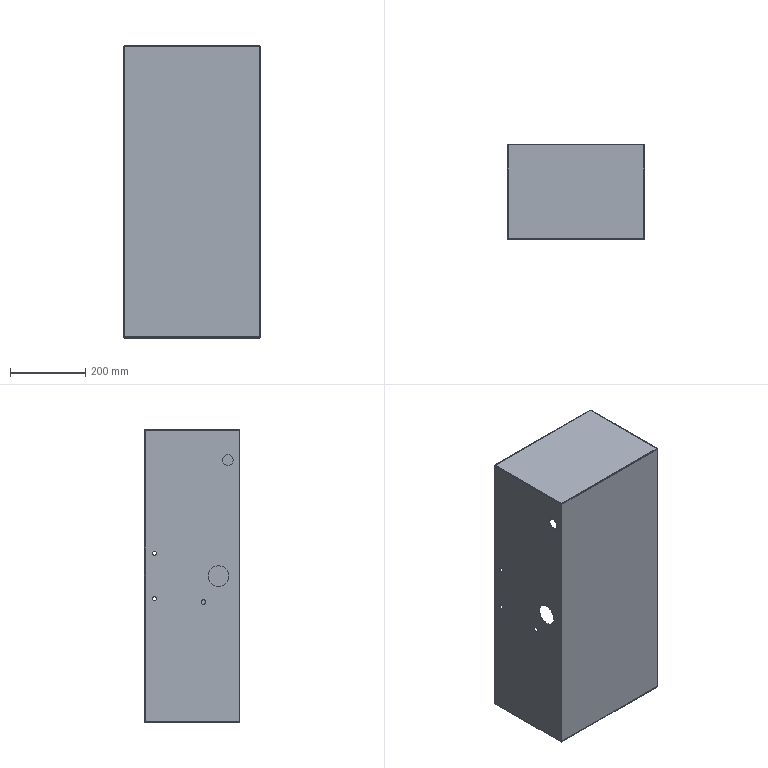Part | SolidWorks | features ICE 8, EdgeFlange 4, 3DProfileFeature 3, HoleWzd 3, FlatPattern 1, SMBaseFlange 1, SheetMetal 1 | 1 solid | 96 faces | box 362.4 x 253.2 x 776.2 mm | volume 1035495 mm3 | plane 48 | cylinder 40 | spline 8 | commonest cylinder face diameters 1 x8 3.4 x8 11 x8 20 x6 10.5 x4 12.5 x2